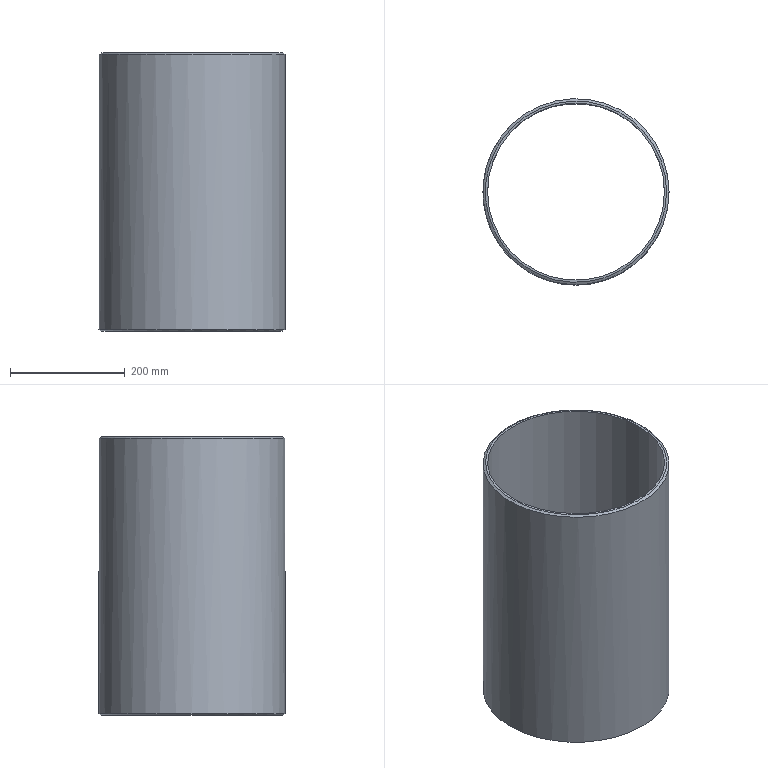Part | NX | features CHAMFER 1, CYLINDER 1, DATUM_CSYS 1, SHELL 1 | 1 solid | 6 faces | box 325 x 325 x 486 mm | volume 3861046 mm3 | plane 2 | cylinder 2 | cone 2 | commonest cylinder face diameters 309 x1 325 x1
STEP:
#1=CARTESIAN_POINT('',(158.17,0.,486.));
#2=VERTEX_POINT('',#1);
#3=CARTESIAN_POINT('',(0.,0.,486.));
#4=DIRECTION('',(0.,0.,1.));
#5=DIRECTION('',(1.,0.,0.));
#6=AXIS2_PLACEMENT_3D('',#3,#4,#5);
#7=CIRCLE('',#6,158.17);
#8=EDGE_CURVE('',#2,#2,#7,.T.);
#9=ORIENTED_EDGE('',*,*,#8,.T.);
#10=EDGE_LOOP('',(#9));
#11=FACE_BOUND('',#10,.T.);
#12=CARTESIAN_POINT('',(154.5,0.,486.));
#13=VERTEX_POINT('',#12);
#14=CARTESIAN_POINT('',(0.,0.,486.));
#15=DIRECTION('',(0.,0.,1.));
#16=DIRECTION('',(1.,0.,0.));
#17=AXIS2_PLACEMENT_3D('',#14,#15,#16);
#18=CIRCLE('',#17,154.5);
#19=EDGE_CURVE('',#13,#13,#18,.F.);
#20=ORIENTED_EDGE('',*,*,#19,.T.);
#21=EDGE_LOOP('',(#20));
#22=FACE_BOUND('',#21,.T.);
#23=CARTESIAN_POINT('',(0.,0.,486.));
#24=DIRECTION('',(0.,0.,1.));
#25=DIRECTION('',(1.,0.,0.));
#26=AXIS2_PLACEMENT_3D('',#23,#24,#25);
#27=PLANE('',#26);
#28=ADVANCED_FACE('',(#11,#22),#27,.T.);
#29=CARTESIAN_POINT('',(-158.17,0.,0.));
#30=VERTEX_POINT('',#29);
#31=CARTESIAN_POINT('',(0.,0.,0.));
#32=DIRECTION('',(0.,0.,-1.));
#33=DIRECTION('',(-1.,0.,0.));
#34=AXIS2_PLACEMENT_3D('',#31,#32,#33);
#35=CIRCLE('',#34,158.17);
#36=EDGE_CURVE('',#30,#30,#35,.T.);
#37=ORIENTED_EDGE('',*,*,#36,.T.);
#38=EDGE_LOOP('',(#37));
#39=FACE_BOUND('',#38,.T.);
#40=CARTESIAN_POINT('',(-154.5,0.,0.));
#41=VERTEX_POINT('',#40);
#42=CARTESIAN_POINT('',(0.,0.,0.));
#43=DIRECTION('',(0.,0.,-1.));
#44=DIRECTION('',(-1.,0.,0.));
#45=AXIS2_PLACEMENT_3D('',#42,#43,#44);
#46=CIRCLE('',#45,154.5);
#47=EDGE_CURVE('',#41,#41,#46,.F.);
#48=ORIENTED_EDGE('',*,*,#47,.T.);
#49=EDGE_LOOP('',(#48));
#50=FACE_BOUND('',#49,.T.);
#51=CARTESIAN_POINT('',(0.,0.,0.));
#52=DIRECTION('',(0.,0.,-1.));
#53=DIRECTION('',(-1.,0.,0.));
#54=AXIS2_PLACEMENT_3D('',#51,#52,#53);
#55=PLANE('',#54);
#56=ADVANCED_FACE('',(#39,#50),#55,.T.);
#57=CARTESIAN_POINT('',(-162.5,0.,2.5));
#58=VERTEX_POINT('',#57);
#59=CARTESIAN_POINT('',(0.,0.,2.5));
#60=DIRECTION('',(0.,0.,-1.));
#61=DIRECTION('',(-1.,0.,0.));
#62=AXIS2_PLACEMENT_3D('',#59,#60,#61);
#63=CIRCLE('',#62,162.5);
#64=EDGE_CURVE('',#58,#58,#63,.F.);
#65=ORIENTED_EDGE('',*,*,#64,.T.);
#66=EDGE_LOOP('',(#65));
#67=FACE_BOUND('',#66,.T.);
#68=CARTESIAN_POINT('',(162.5,0.,483.5));
#69=VERTEX_POINT('',#68);
#70=CARTESIAN_POINT('',(0.,0.,483.5));
#71=DIRECTION('',(0.,0.,1.));
#72=DIRECTION('',(1.,0.,0.));
#73=AXIS2_PLACEMENT_3D('',#70,#71,#72);
#74=CIRCLE('',#73,162.5);
#75=EDGE_CURVE('',#69,#69,#74,.F.);
#76=ORIENTED_EDGE('',*,*,#75,.T.);
#77=EDGE_LOOP('',(#76));
#78=FACE_BOUND('',#77,.T.);
#79=CARTESIAN_POINT('',(0.,0.,0.));
#80=DIRECTION('',(0.,0.,1.));
#81=DIRECTION('',(1.,0.,0.));
#82=AXIS2_PLACEMENT_3D('',#79,#80,#81);
#83=CYLINDRICAL_SURFACE('',#82,162.5);
#84=ADVANCED_FACE('',(#67,#78),#83,.T.);
#85=ORIENTED_EDGE('',*,*,#19,.F.);
#86=EDGE_LOOP('',(#85));
#87=FACE_BOUND('',#86,.T.);
#88=ORIENTED_EDGE('',*,*,#47,.F.);
#89=EDGE_LOOP('',(#88));
#90=FACE_BOUND('',#89,.T.);
#91=CARTESIAN_POINT('',(0.,0.,0.));
#92=DIRECTION('',(0.,0.,1.));
#93=DIRECTION('',(1.,0.,0.));
#94=AXIS2_PLACEMENT_3D('',#91,#92,#93);
#95=CYLINDRICAL_SURFACE('',#94,154.5);
#96=ADVANCED_FACE('',(#87,#90),#95,.F.);
#97=ORIENTED_EDGE('',*,*,#36,.F.);
#98=EDGE_LOOP('',(#97));
#99=FACE_BOUND('',#98,.T.);
#100=ORIENTED_EDGE('',*,*,#64,.F.);
#101=EDGE_LOOP('',(#100));
#102=FACE_BOUND('',#101,.T.);
#103=CARTESIAN_POINT('',(0.,0.,2.5));
#104=DIRECTION('',(0.,0.,1.));
#105=DIRECTION('',(1.,0.,0.));
#106=AXIS2_PLACEMENT_3D('',#103,#104,#105);
#107=CONICAL_SURFACE('',#106,162.5,1.047);
#108=ADVANCED_FACE('',(#99,#102),#107,.T.);
#109=ORIENTED_EDGE('',*,*,#8,.F.);
#110=EDGE_LOOP('',(#109));
#111=FACE_BOUND('',#110,.T.);
#112=ORIENTED_EDGE('',*,*,#75,.F.);
#113=EDGE_LOOP('',(#112));
#114=FACE_BOUND('',#113,.T.);
#115=CARTESIAN_POINT('',(0.,0.,483.5));
#116=DIRECTION('',(0.,0.,-1.));
#117=DIRECTION('',(-1.,0.,0.));
#118=AXIS2_PLACEMENT_3D('',#115,#116,#117);
#119=CONICAL_SURFACE('',#118,162.5,1.047);
#120=ADVANCED_FACE('',(#111,#114),#119,.T.);
#121=CLOSED_SHELL('',(#28,#56,#84,#96,#108,#120));
#122=MANIFOLD_SOLID_BREP('',#121);
#123=(LENGTH_UNIT()NAMED_UNIT(*)SI_UNIT(.MILLI.,.METRE.));
#124=UNCERTAINTY_MEASURE_WITH_UNIT(LENGTH_MEASURE(0.00001),#123,'','');
#125=(NAMED_UNIT(*)PLANE_ANGLE_UNIT()SI_UNIT($,.RADIAN.));
#126=(NAMED_UNIT(*)SI_UNIT($,.STERADIAN.)SOLID_ANGLE_UNIT());
#127=(GEOMETRIC_REPRESENTATION_CONTEXT(3)GLOBAL_UNCERTAINTY_ASSIGNED_CONTEXT((#124))GLOBAL_UNIT_ASSIGNED_CONTEXT((#123,#125,#126))REPRESENTATION_CONTEXT('',''));
#128=ADVANCED_BREP_SHAPE_REPRESENTATION('',(#122),#127);